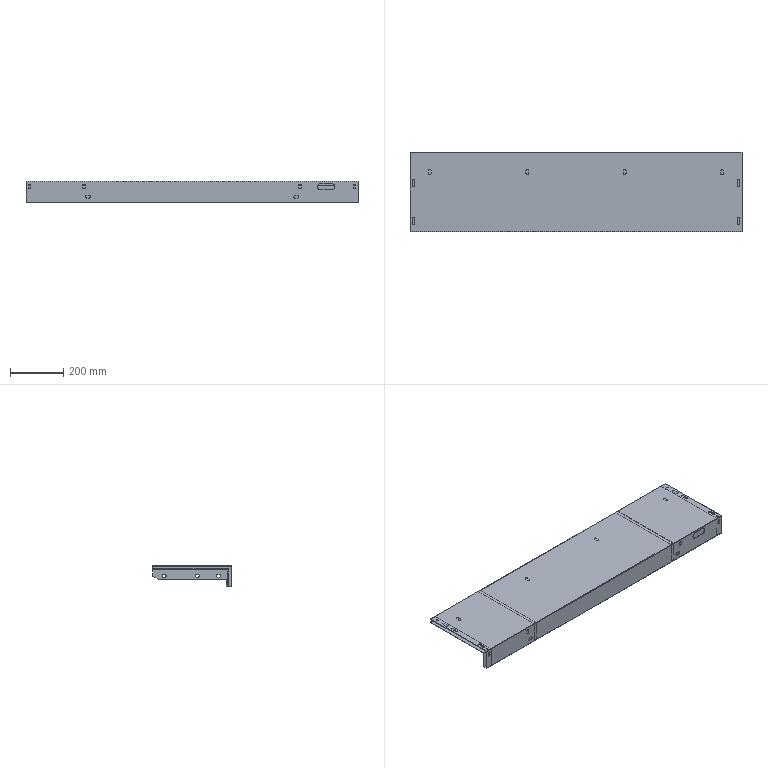Part | SolidWorks | 6 solids | 360 faces | box 1250 x 299.8 x 80.3 mm | volume 1285406 mm3 | plane 230 | cylinder 130 | commonest cylinder face diameters 6 x45 10 x32 9 x20 11 x10 0.4 x8 2.4 x5